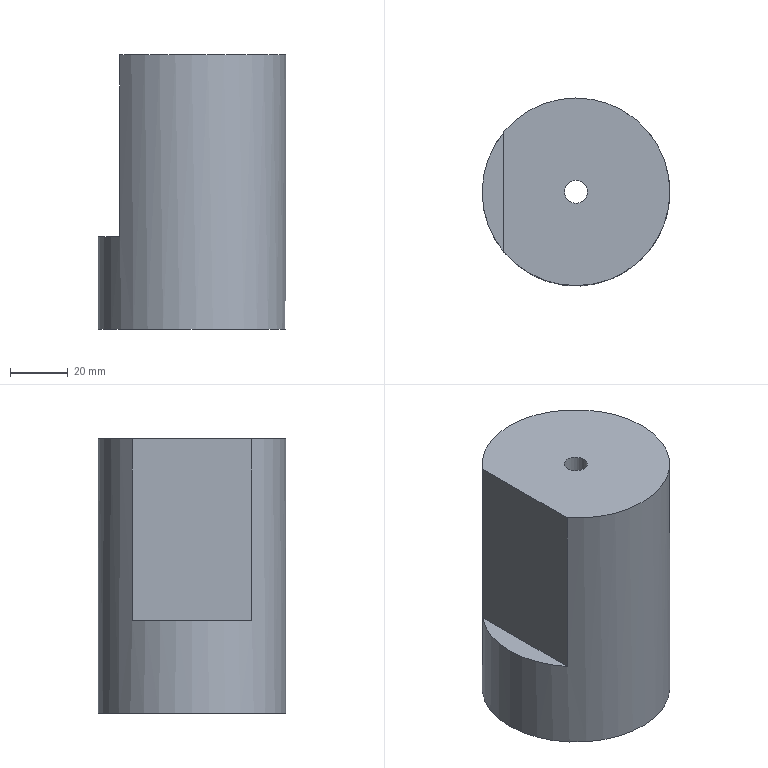Part | NX | features solid 2 | 1 solid | 8 faces | box 65 x 65 x 95 mm | volume 214799 mm3 | plane 5 | cylinder 3 | commonest cylinder face diameters 8 x1 36 x1 65 x1
STEP:
#1=CARTESIAN_POINT('',(-625.,-50.767,-54.));
#2=VERTEX_POINT('',#1);
#3=CARTESIAN_POINT('',(-625.,-9.233,-54.));
#4=VERTEX_POINT('',#3);
#5=CARTESIAN_POINT('',(-600.,-30.,-54.));
#6=DIRECTION('',(0.,0.,-1.));
#7=DIRECTION('',(-1.,0.,0.));
#8=AXIS2_PLACEMENT_3D('',#5,#6,#7);
#9=CIRCLE('',#8,32.5);
#10=EDGE_CURVE('',#2,#4,#9,.F.);
#11=ORIENTED_EDGE('',*,*,#10,.F.);
#12=CARTESIAN_POINT('',(-625.,-50.767,-117.));
#13=VERTEX_POINT('',#12);
#14=CARTESIAN_POINT('',(-625.,-50.767,-42.));
#15=DIRECTION('',(0.,0.,-1.));
#16=VECTOR('',#15,1000.);
#17=LINE('',#14,#16);
#18=EDGE_CURVE('',#2,#13,#17,.T.);
#19=ORIENTED_EDGE('',*,*,#18,.T.);
#20=CARTESIAN_POINT('',(-625.,-9.233,-117.));
#21=VERTEX_POINT('',#20);
#22=CARTESIAN_POINT('',(-600.,-30.,-117.));
#23=DIRECTION('',(0.,0.,1.));
#24=DIRECTION('',(1.,0.,0.));
#25=AXIS2_PLACEMENT_3D('',#22,#23,#24);
#26=CIRCLE('',#25,32.5);
#27=EDGE_CURVE('',#13,#21,#26,.F.);
#28=ORIENTED_EDGE('',*,*,#27,.T.);
#29=CARTESIAN_POINT('',(-625.,-9.233,-42.));
#30=DIRECTION('',(0.,0.,-1.));
#31=VECTOR('',#30,1000.);
#32=LINE('',#29,#31);
#33=EDGE_CURVE('',#21,#4,#32,.F.);
#34=ORIENTED_EDGE('',*,*,#33,.T.);
#35=EDGE_LOOP('',(#11,#19,#28,#34));
#36=FACE_BOUND('',#35,.T.);
#37=CARTESIAN_POINT('',(-632.5,-30.,-149.));
#38=VERTEX_POINT('',#37);
#39=CARTESIAN_POINT('',(-600.,-30.,-149.));
#40=DIRECTION('',(0.,0.,-1.));
#41=DIRECTION('',(-1.,0.,0.));
#42=AXIS2_PLACEMENT_3D('',#39,#40,#41);
#43=CIRCLE('',#42,32.5);
#44=EDGE_CURVE('',#38,#38,#43,.F.);
#45=ORIENTED_EDGE('',*,*,#44,.T.);
#46=EDGE_LOOP('',(#45));
#47=FACE_BOUND('',#46,.T.);
#48=CARTESIAN_POINT('',(-600.,-30.,-42.));
#49=DIRECTION('',(0.,0.,-1.));
#50=DIRECTION('',(-1.,0.,0.));
#51=AXIS2_PLACEMENT_3D('',#48,#49,#50);
#52=CYLINDRICAL_SURFACE('',#51,32.5);
#53=ADVANCED_FACE('',(#36,#47),#52,.T.);
#54=CARTESIAN_POINT('',(-596.,-30.,-54.));
#55=VERTEX_POINT('',#54);
#56=CARTESIAN_POINT('',(-600.,-30.,-54.));
#57=DIRECTION('',(0.,0.,1.));
#58=DIRECTION('',(1.,0.,0.));
#59=AXIS2_PLACEMENT_3D('',#56,#57,#58);
#60=CIRCLE('',#59,4.);
#61=EDGE_CURVE('',#55,#55,#60,.T.);
#62=ORIENTED_EDGE('',*,*,#61,.F.);
#63=EDGE_LOOP('',(#62));
#64=FACE_BOUND('',#63,.T.);
#65=CARTESIAN_POINT('',(-625.,-70.,-54.));
#66=DIRECTION('',(0.,1.,0.));
#67=VECTOR('',#66,1000.);
#68=LINE('',#65,#67);
#69=EDGE_CURVE('',#2,#4,#68,.T.);
#70=ORIENTED_EDGE('',*,*,#69,.F.);
#71=ORIENTED_EDGE('',*,*,#10,.T.);
#72=EDGE_LOOP('',(#70,#71));
#73=FACE_BOUND('',#72,.T.);
#74=CARTESIAN_POINT('',(-600.,-30.,-54.));
#75=DIRECTION('',(0.,0.,1.));
#76=DIRECTION('',(1.,0.,0.));
#77=AXIS2_PLACEMENT_3D('',#74,#75,#76);
#78=PLANE('',#77);
#79=ADVANCED_FACE('',(#64,#73),#78,.T.);
#80=CARTESIAN_POINT('',(-618.,-30.,-149.));
#81=VERTEX_POINT('',#80);
#82=CARTESIAN_POINT('',(-600.,-30.,-149.));
#83=DIRECTION('',(0.,0.,-1.));
#84=DIRECTION('',(-1.,0.,0.));
#85=AXIS2_PLACEMENT_3D('',#82,#83,#84);
#86=CIRCLE('',#85,18.);
#87=EDGE_CURVE('',#81,#81,#86,.T.);
#88=ORIENTED_EDGE('',*,*,#87,.F.);
#89=EDGE_LOOP('',(#88));
#90=FACE_BOUND('',#89,.T.);
#91=ORIENTED_EDGE('',*,*,#44,.F.);
#92=EDGE_LOOP('',(#91));
#93=FACE_BOUND('',#92,.T.);
#94=CARTESIAN_POINT('',(-600.,-30.,-149.));
#95=DIRECTION('',(0.,0.,1.));
#96=DIRECTION('',(1.,0.,0.));
#97=AXIS2_PLACEMENT_3D('',#94,#95,#96);
#98=PLANE('',#97);
#99=ADVANCED_FACE('',(#90,#93),#98,.F.);
#100=CARTESIAN_POINT('',(-625.,-70.,-117.));
#101=DIRECTION('',(0.,1.,0.));
#102=VECTOR('',#101,1000.);
#103=LINE('',#100,#102);
#104=EDGE_CURVE('',#13,#21,#103,.T.);
#105=ORIENTED_EDGE('',*,*,#104,.T.);
#106=ORIENTED_EDGE('',*,*,#27,.F.);
#107=EDGE_LOOP('',(#105,#106));
#108=FACE_BOUND('',#107,.T.);
#109=CARTESIAN_POINT('',(-625.,-70.,-117.));
#110=DIRECTION('',(0.,0.,-1.));
#111=DIRECTION('',(0.,1.,0.));
#112=AXIS2_PLACEMENT_3D('',#109,#110,#111);
#113=PLANE('',#112);
#114=ADVANCED_FACE('',(#108),#113,.F.);
#115=ORIENTED_EDGE('',*,*,#69,.T.);
#116=ORIENTED_EDGE('',*,*,#33,.F.);
#117=ORIENTED_EDGE('',*,*,#104,.F.);
#118=ORIENTED_EDGE('',*,*,#18,.F.);
#119=EDGE_LOOP('',(#115,#116,#117,#118));
#120=FACE_BOUND('',#119,.T.);
#121=CARTESIAN_POINT('',(-625.,-70.,-52.));
#122=DIRECTION('',(1.,0.,0.));
#123=DIRECTION('',(0.,0.,-1.));
#124=AXIS2_PLACEMENT_3D('',#121,#122,#123);
#125=PLANE('',#124);
#126=ADVANCED_FACE('',(#120),#125,.F.);
#127=CARTESIAN_POINT('',(-618.,-30.,-64.));
#128=VERTEX_POINT('',#127);
#129=CARTESIAN_POINT('',(-600.,-30.,-64.));
#130=DIRECTION('',(0.,0.,-1.));
#131=DIRECTION('',(-1.,0.,0.));
#132=AXIS2_PLACEMENT_3D('',#129,#130,#131);
#133=CIRCLE('',#132,18.);
#134=EDGE_CURVE('',#128,#128,#133,.T.);
#135=ORIENTED_EDGE('',*,*,#134,.F.);
#136=EDGE_LOOP('',(#135));
#137=FACE_BOUND('',#136,.T.);
#138=ORIENTED_EDGE('',*,*,#87,.T.);
#139=EDGE_LOOP('',(#138));
#140=FACE_BOUND('',#139,.T.);
#141=CARTESIAN_POINT('',(-600.,-30.,-214.));
#142=DIRECTION('',(0.,0.,1.));
#143=DIRECTION('',(-1.,0.,0.));
#144=AXIS2_PLACEMENT_3D('',#141,#142,#143);
#145=CYLINDRICAL_SURFACE('',#144,18.);
#146=ADVANCED_FACE('',(#137,#140),#145,.F.);
#147=CARTESIAN_POINT('',(-596.,-30.,-64.));
#148=VERTEX_POINT('',#147);
#149=CARTESIAN_POINT('',(-600.,-30.,-64.));
#150=DIRECTION('',(0.,0.,1.));
#151=DIRECTION('',(1.,0.,0.));
#152=AXIS2_PLACEMENT_3D('',#149,#150,#151);
#153=CIRCLE('',#152,4.);
#154=EDGE_CURVE('',#148,#148,#153,.T.);
#155=ORIENTED_EDGE('',*,*,#154,.T.);
#156=EDGE_LOOP('',(#155));
#157=FACE_BOUND('',#156,.T.);
#158=ORIENTED_EDGE('',*,*,#134,.T.);
#159=EDGE_LOOP('',(#158));
#160=FACE_BOUND('',#159,.T.);
#161=CARTESIAN_POINT('',(-600.,-30.,-64.));
#162=DIRECTION('',(0.,0.,1.));
#163=DIRECTION('',(1.,0.,0.));
#164=AXIS2_PLACEMENT_3D('',#161,#162,#163);
#165=PLANE('',#164);
#166=ADVANCED_FACE('',(#157,#160),#165,.F.);
#167=ORIENTED_EDGE('',*,*,#61,.T.);
#168=EDGE_LOOP('',(#167));
#169=FACE_BOUND('',#168,.T.);
#170=ORIENTED_EDGE('',*,*,#154,.F.);
#171=EDGE_LOOP('',(#170));
#172=FACE_BOUND('',#171,.T.);
#173=CARTESIAN_POINT('',(-600.,-30.,-104.));
#174=DIRECTION('',(0.,0.,1.));
#175=DIRECTION('',(1.,0.,0.));
#176=AXIS2_PLACEMENT_3D('',#173,#174,#175);
#177=CYLINDRICAL_SURFACE('',#176,4.);
#178=ADVANCED_FACE('',(#169,#172),#177,.F.);
#179=CLOSED_SHELL('',(#53,#79,#99,#114,#126,#146,#166,#178));
#180=MANIFOLD_SOLID_BREP('',#179);
#181=(LENGTH_UNIT()NAMED_UNIT(*)SI_UNIT(.MILLI.,.METRE.));
#182=UNCERTAINTY_MEASURE_WITH_UNIT(LENGTH_MEASURE(0.00001),#181,'','');
#183=(NAMED_UNIT(*)PLANE_ANGLE_UNIT()SI_UNIT($,.RADIAN.));
#184=(NAMED_UNIT(*)SI_UNIT($,.STERADIAN.)SOLID_ANGLE_UNIT());
#185=(GEOMETRIC_REPRESENTATION_CONTEXT(3)GLOBAL_UNCERTAINTY_ASSIGNED_CONTEXT((#182))GLOBAL_UNIT_ASSIGNED_CONTEXT((#181,#183,#184))REPRESENTATION_CONTEXT('',''));
#186=ADVANCED_BREP_SHAPE_REPRESENTATION('',(#180),#185);